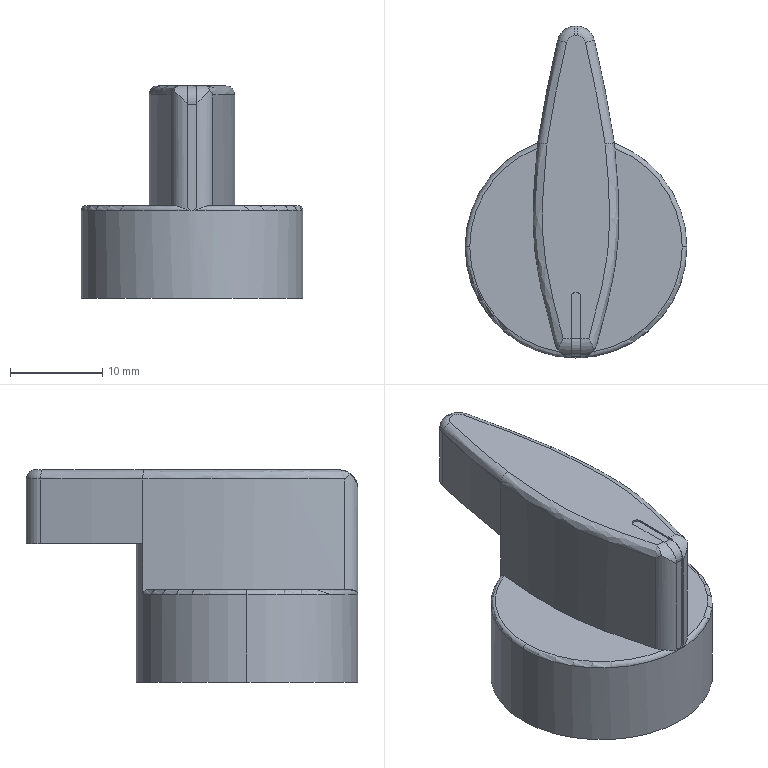Part | STEP file | Switch CR-253 | 1 solid | 38 faces | box 24 x 35.897 x 23 mm | volume 7467 mm3 | cylinder 12 | torus 9 | plane 9 | spline 8 | commonest cylinder face diameters 1 x4 4 x4 24 x2 3.092 x1 5.11 x1